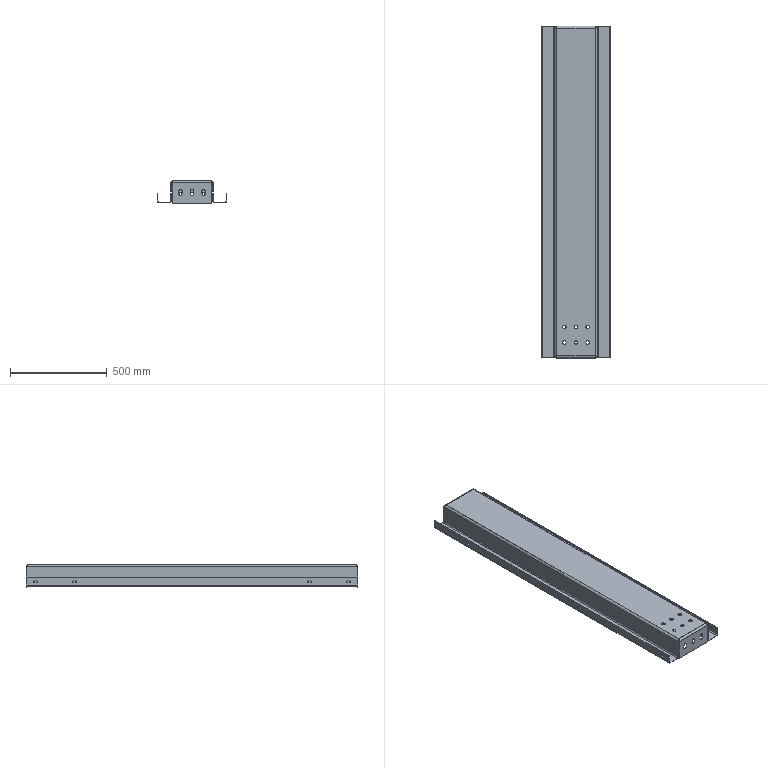Part | STEP file | SYL_0392D6J1SYL0380DJ100-509338 | 1 solid | 138 faces | box 360 x 1720 x 116 mm | volume 2326714 mm3 | plane 68 | cylinder 62 | spline 8 | commonest cylinder face diameters 18 x34 10 x20 14 x4 22 x4